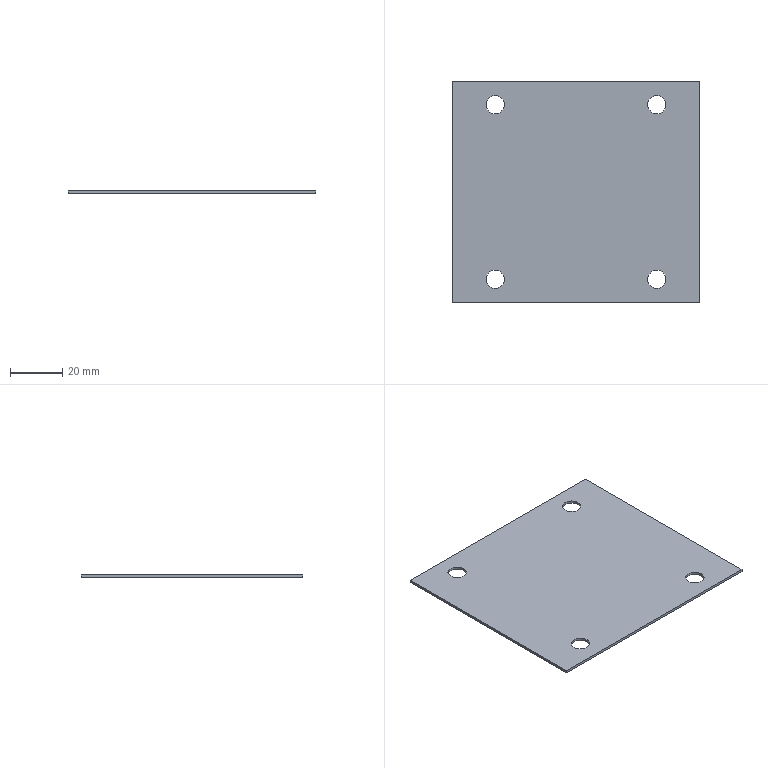Part | STEP file | GLSJ-10-45 | 1 solid | 14 faces | box 95 x 85 x 1 mm | volume 7921 mm3 | cylinder 8 | plane 6 | commonest cylinder face diameters 7 x8
STEP:
#1=CARTESIAN_POINT('',(0.,0.,0.));
#2=DIRECTION('',(0.,0.,1.));
#3=DIRECTION('',(1.,0.,0.));
#4=AXIS2_PLACEMENT_3D('',#1,#2,#3);
#5=CARTESIAN_POINT('',(-27.5,-33.5,0.));
#6=VERTEX_POINT('',#5);
#7=CARTESIAN_POINT('',(-27.5,-33.5,1.));
#8=VERTEX_POINT('',#7);
#9=CARTESIAN_POINT('',(-27.5,-33.5,0.));
#10=DIRECTION('',(0.,0.,1.));
#11=VECTOR('',#10,1.);
#12=LINE('',#9,#11);
#13=CARTESIAN_POINT('',(-31.,-33.5,0.));
#14=DIRECTION('',(0.,0.,1.));
#15=DIRECTION('',(1.,0.,0.));
#16=AXIS2_PLACEMENT_3D('',#13,#14,#15);
#17=CYLINDRICAL_SURFACE('',#16,3.5);
#18=CARTESIAN_POINT('',(6.283,0.));
#19=DIRECTION('',(0.,1.));
#20=VECTOR('',#19,1.);
#21=LINE('',#18,#20);
#22=(GEOMETRIC_REPRESENTATION_CONTEXT(2)PARAMETRIC_REPRESENTATION_CONTEXT()REPRESENTATION_CONTEXT('',''));
#23=DEFINITIONAL_REPRESENTATION('',(#21),#22);
#24=PCURVE('',#17,#23);
#25=CARTESIAN_POINT('',(-31.,-33.5,0.));
#26=DIRECTION('',(0.,0.,1.));
#27=DIRECTION('',(1.,0.,0.));
#28=AXIS2_PLACEMENT_3D('',#25,#26,#27);
#29=CYLINDRICAL_SURFACE('',#28,3.5);
#30=CARTESIAN_POINT('',(0.,0.));
#31=DIRECTION('',(0.,1.));
#32=VECTOR('',#31,1.);
#33=LINE('',#30,#32);
#34=(GEOMETRIC_REPRESENTATION_CONTEXT(2)PARAMETRIC_REPRESENTATION_CONTEXT()REPRESENTATION_CONTEXT('',''));
#35=DEFINITIONAL_REPRESENTATION('',(#33),#34);
#36=PCURVE('',#29,#35);
#37=SURFACE_CURVE('',#12,(#24,#36),.PCURVE_S1.);
#38=EDGE_CURVE('',#6,#8,#37,.T.);
#39=ORIENTED_EDGE('',*,*,#38,.T.);
#40=CARTESIAN_POINT('',(-34.5,-33.5,1.));
#41=VERTEX_POINT('',#40);
#42=CARTESIAN_POINT('',(-31.,-33.5,1.));
#43=DIRECTION('',(0.,0.,1.));
#44=DIRECTION('',(-1.,0.,0.));
#45=AXIS2_PLACEMENT_3D('',#42,#43,#44);
#46=CIRCLE('',#45,3.5);
#47=CARTESIAN_POINT('',(3.142,1.));
#48=DIRECTION('',(1.,0.));
#49=VECTOR('',#48,1.);
#50=LINE('',#47,#49);
#51=(GEOMETRIC_REPRESENTATION_CONTEXT(2)PARAMETRIC_REPRESENTATION_CONTEXT()REPRESENTATION_CONTEXT('',''));
#52=DEFINITIONAL_REPRESENTATION('',(#50),#51);
#53=PCURVE('',#17,#52);
#54=CARTESIAN_POINT('',(0.,0.,1.));
#55=DIRECTION('',(0.,0.,-1.));
#56=DIRECTION('',(-1.,0.,0.));
#57=AXIS2_PLACEMENT_3D('',#54,#55,#56);
#58=PLANE('',#57);
#59=CARTESIAN_POINT('',(34.5,-33.5));
#60=CARTESIAN_POINT('',(34.5,-39.562));
#61=CARTESIAN_POINT('',(29.25,-36.531));
#62=CARTESIAN_POINT('',(24.,-33.5));
#63=CARTESIAN_POINT('',(29.25,-30.469));
#64=CARTESIAN_POINT('',(34.5,-27.438));
#65=CARTESIAN_POINT('',(34.5,-33.5));
#66=(BOUNDED_CURVE()B_SPLINE_CURVE(2,(#59,#60,#61,#62,#63,#64,#65),.UNSPECIFIED.,.T.,.F.)B_SPLINE_CURVE_WITH_KNOTS((1,2,2,2,2,1),(-2.094,0.,2.094,4.189,6.283,8.378),.UNSPECIFIED.)CURVE()GEOMETRIC_REPRESENTATION_ITEM()RATIONAL_B_SPLINE_CURVE((1.,0.5,1.,0.5,1.,0.5,1.))REPRESENTATION_ITEM(''));
#67=(GEOMETRIC_REPRESENTATION_CONTEXT(2)PARAMETRIC_REPRESENTATION_CONTEXT()REPRESENTATION_CONTEXT('',''));
#68=DEFINITIONAL_REPRESENTATION('',(#66),#67);
#69=PCURVE('',#58,#68);
#70=SURFACE_CURVE('',#46,(#53,#69),.PCURVE_S1.);
#71=EDGE_CURVE('',#41,#8,#70,.T.);
#72=ORIENTED_EDGE('',*,*,#71,.F.);
#73=CARTESIAN_POINT('',(-34.5,-33.5,0.));
#74=VERTEX_POINT('',#73);
#75=CARTESIAN_POINT('',(-34.5,-33.5,0.));
#76=DIRECTION('',(0.,0.,1.));
#77=VECTOR('',#76,1.);
#78=LINE('',#75,#77);
#79=CARTESIAN_POINT('',(3.142,0.));
#80=DIRECTION('',(0.,1.));
#81=VECTOR('',#80,1.);
#82=LINE('',#79,#81);
#83=(GEOMETRIC_REPRESENTATION_CONTEXT(2)PARAMETRIC_REPRESENTATION_CONTEXT()REPRESENTATION_CONTEXT('',''));
#84=DEFINITIONAL_REPRESENTATION('',(#82),#83);
#85=PCURVE('',#17,#84);
#86=CARTESIAN_POINT('',(3.142,0.));
#87=DIRECTION('',(0.,1.));
#88=VECTOR('',#87,1.);
#89=LINE('',#86,#88);
#90=(GEOMETRIC_REPRESENTATION_CONTEXT(2)PARAMETRIC_REPRESENTATION_CONTEXT()REPRESENTATION_CONTEXT('',''));
#91=DEFINITIONAL_REPRESENTATION('',(#89),#90);
#92=PCURVE('',#29,#91);
#93=SURFACE_CURVE('',#78,(#85,#92),.PCURVE_S1.);
#94=EDGE_CURVE('',#74,#41,#93,.T.);
#95=ORIENTED_EDGE('',*,*,#94,.F.);
#96=CARTESIAN_POINT('',(-31.,-33.5,0.));
#97=DIRECTION('',(0.,0.,1.));
#98=DIRECTION('',(-1.,0.,0.));
#99=AXIS2_PLACEMENT_3D('',#96,#97,#98);
#100=CIRCLE('',#99,3.5);
#101=CARTESIAN_POINT('',(3.142,0.));
#102=DIRECTION('',(1.,0.));
#103=VECTOR('',#102,1.);
#104=LINE('',#101,#103);
#105=(GEOMETRIC_REPRESENTATION_CONTEXT(2)PARAMETRIC_REPRESENTATION_CONTEXT()REPRESENTATION_CONTEXT('',''));
#106=DEFINITIONAL_REPRESENTATION('',(#104),#105);
#107=PCURVE('',#17,#106);
#108=CARTESIAN_POINT('',(0.,0.,0.));
#109=DIRECTION('',(0.,0.,-1.));
#110=DIRECTION('',(-1.,0.,0.));
#111=AXIS2_PLACEMENT_3D('',#108,#109,#110);
#112=PLANE('',#111);
#113=CARTESIAN_POINT('',(34.5,-33.5));
#114=CARTESIAN_POINT('',(34.5,-39.562));
#115=CARTESIAN_POINT('',(29.25,-36.531));
#116=CARTESIAN_POINT('',(24.,-33.5));
#117=CARTESIAN_POINT('',(29.25,-30.469));
#118=CARTESIAN_POINT('',(34.5,-27.438));
#119=CARTESIAN_POINT('',(34.5,-33.5));
#120=(BOUNDED_CURVE()B_SPLINE_CURVE(2,(#113,#114,#115,#116,#117,#118,#119),.UNSPECIFIED.,.T.,.F.)B_SPLINE_CURVE_WITH_KNOTS((1,2,2,2,2,1),(-2.094,0.,2.094,4.189,6.283,8.378),.UNSPECIFIED.)CURVE()GEOMETRIC_REPRESENTATION_ITEM()RATIONAL_B_SPLINE_CURVE((1.,0.5,1.,0.5,1.,0.5,1.))REPRESENTATION_ITEM(''));
#121=(GEOMETRIC_REPRESENTATION_CONTEXT(2)PARAMETRIC_REPRESENTATION_CONTEXT()REPRESENTATION_CONTEXT('',''));
#122=DEFINITIONAL_REPRESENTATION('',(#120),#121);
#123=PCURVE('',#112,#122);
#124=SURFACE_CURVE('',#100,(#107,#123),.PCURVE_S1.);
#125=EDGE_CURVE('',#74,#6,#124,.T.);
#126=ORIENTED_EDGE('',*,*,#125,.T.);
#127=EDGE_LOOP('',(#39,#72,#95,#126));
#128=FACE_BOUND('',#127,.F.);
#129=ADVANCED_FACE('',(#128),#17,.F.);
#130=CARTESIAN_POINT('',(34.5,-33.5,0.));
#131=VERTEX_POINT('',#130);
#132=CARTESIAN_POINT('',(34.5,-33.5,1.));
#133=VERTEX_POINT('',#132);
#134=CARTESIAN_POINT('',(34.5,-33.5,0.));
#135=DIRECTION('',(0.,0.,1.));
#136=VECTOR('',#135,1.);
#137=LINE('',#134,#136);
#138=CARTESIAN_POINT('',(31.,-33.5,0.));
#139=DIRECTION('',(0.,0.,1.));
#140=DIRECTION('',(1.,0.,0.));
#141=AXIS2_PLACEMENT_3D('',#138,#139,#140);
#142=CYLINDRICAL_SURFACE('',#141,3.5);
#143=CARTESIAN_POINT('',(6.283,0.));
#144=DIRECTION('',(0.,1.));
#145=VECTOR('',#144,1.);
#146=LINE('',#143,#145);
#147=(GEOMETRIC_REPRESENTATION_CONTEXT(2)PARAMETRIC_REPRESENTATION_CONTEXT()REPRESENTATION_CONTEXT('',''));
#148=DEFINITIONAL_REPRESENTATION('',(#146),#147);
#149=PCURVE('',#142,#148);
#150=CARTESIAN_POINT('',(31.,-33.5,0.));
#151=DIRECTION('',(0.,0.,1.));
#152=DIRECTION('',(1.,0.,0.));
#153=AXIS2_PLACEMENT_3D('',#150,#151,#152);
#154=CYLINDRICAL_SURFACE('',#153,3.5);
#155=CARTESIAN_POINT('',(0.,0.));
#156=DIRECTION('',(0.,1.));
#157=VECTOR('',#156,1.);
#158=LINE('',#155,#157);
#159=(GEOMETRIC_REPRESENTATION_CONTEXT(2)PARAMETRIC_REPRESENTATION_CONTEXT()REPRESENTATION_CONTEXT('',''));
#160=DEFINITIONAL_REPRESENTATION('',(#158),#159);
#161=PCURVE('',#154,#160);
#162=SURFACE_CURVE('',#137,(#149,#161),.PCURVE_S1.);
#163=EDGE_CURVE('',#131,#133,#162,.T.);
#164=ORIENTED_EDGE('',*,*,#163,.T.);
#165=CARTESIAN_POINT('',(27.5,-33.5,1.));
#166=VERTEX_POINT('',#165);
#167=CARTESIAN_POINT('',(31.,-33.5,1.));
#168=DIRECTION('',(0.,0.,1.));
#169=DIRECTION('',(1.,0.,0.));
#170=AXIS2_PLACEMENT_3D('',#167,#168,#169);
#171=CIRCLE('',#170,3.5);
#172=CARTESIAN_POINT('',(0.,1.));
#173=DIRECTION('',(1.,0.));
#174=VECTOR('',#173,1.);
#175=LINE('',#172,#174);
#176=(GEOMETRIC_REPRESENTATION_CONTEXT(2)PARAMETRIC_REPRESENTATION_CONTEXT()REPRESENTATION_CONTEXT('',''));
#177=DEFINITIONAL_REPRESENTATION('',(#175),#176);
#178=PCURVE('',#142,#177);
#179=CARTESIAN_POINT('',(-34.5,-33.5));
#180=CARTESIAN_POINT('',(-34.5,-27.438));
#181=CARTESIAN_POINT('',(-29.25,-30.469));
#182=CARTESIAN_POINT('',(-24.,-33.5));
#183=CARTESIAN_POINT('',(-29.25,-36.531));
#184=CARTESIAN_POINT('',(-34.5,-39.562));
#185=CARTESIAN_POINT('',(-34.5,-33.5));
#186=(BOUNDED_CURVE()B_SPLINE_CURVE(2,(#179,#180,#181,#182,#183,#184,#185),.UNSPECIFIED.,.T.,.F.)B_SPLINE_CURVE_WITH_KNOTS((1,2,2,2,2,1),(-2.094,0.,2.094,4.189,6.283,8.378),.UNSPECIFIED.)CURVE()GEOMETRIC_REPRESENTATION_ITEM()RATIONAL_B_SPLINE_CURVE((1.,0.5,1.,0.5,1.,0.5,1.))REPRESENTATION_ITEM(''));
#187=(GEOMETRIC_REPRESENTATION_CONTEXT(2)PARAMETRIC_REPRESENTATION_CONTEXT()REPRESENTATION_CONTEXT('',''));
#188=DEFINITIONAL_REPRESENTATION('',(#186),#187);
#189=PCURVE('',#58,#188);
#190=SURFACE_CURVE('',#171,(#178,#189),.PCURVE_S1.);
#191=EDGE_CURVE('',#166,#133,#190,.T.);
#192=ORIENTED_EDGE('',*,*,#191,.F.);
#193=CARTESIAN_POINT('',(27.5,-33.5,0.));
#194=VERTEX_POINT('',#193);
#195=CARTESIAN_POINT('',(27.5,-33.5,0.));
#196=DIRECTION('',(0.,0.,1.));
#197=VECTOR('',#196,1.);
#198=LINE('',#195,#197);
#199=CARTESIAN_POINT('',(3.142,0.));
#200=DIRECTION('',(0.,1.));
#201=VECTOR('',#200,1.);
#202=LINE('',#199,#201);
#203=(GEOMETRIC_REPRESENTATION_CONTEXT(2)PARAMETRIC_REPRESENTATION_CONTEXT()REPRESENTATION_CONTEXT('',''));
#204=DEFINITIONAL_REPRESENTATION('',(#202),#203);
#205=PCURVE('',#142,#204);
#206=CARTESIAN_POINT('',(3.142,0.));
#207=DIRECTION('',(0.,1.));
#208=VECTOR('',#207,1.);
#209=LINE('',#206,#208);
#210=(GEOMETRIC_REPRESENTATION_CONTEXT(2)PARAMETRIC_REPRESENTATION_CONTEXT()REPRESENTATION_CONTEXT('',''));
#211=DEFINITIONAL_REPRESENTATION('',(#209),#210);
#212=PCURVE('',#154,#211);
#213=SURFACE_CURVE('',#198,(#205,#212),.PCURVE_S1.);
#214=EDGE_CURVE('',#194,#166,#213,.T.);
#215=ORIENTED_EDGE('',*,*,#214,.F.);
#216=CARTESIAN_POINT('',(31.,-33.5,0.));
#217=DIRECTION('',(0.,0.,1.));
#218=DIRECTION('',(1.,0.,0.));
#219=AXIS2_PLACEMENT_3D('',#216,#217,#218);
#220=CIRCLE('',#219,3.5);
#221=CARTESIAN_POINT('',(0.,0.));
#222=DIRECTION('',(1.,0.));
#223=VECTOR('',#222,1.);
#224=LINE('',#221,#223);
#225=(GEOMETRIC_REPRESENTATION_CONTEXT(2)PARAMETRIC_REPRESENTATION_CONTEXT()REPRESENTATION_CONTEXT('',''));
#226=DEFINITIONAL_REPRESENTATION('',(#224),#225);
#227=PCURVE('',#142,#226);
#228=CARTESIAN_POINT('',(-34.5,-33.5));
#229=CARTESIAN_POINT('',(-34.5,-27.438));
#230=CARTESIAN_POINT('',(-29.25,-30.469));
#231=CARTESIAN_POINT('',(-24.,-33.5));
#232=CARTESIAN_POINT('',(-29.25,-36.531));
#233=CARTESIAN_POINT('',(-34.5,-39.562));
#234=CARTESIAN_POINT('',(-34.5,-33.5));
#235=(BOUNDED_CURVE()B_SPLINE_CURVE(2,(#228,#229,#230,#231,#232,#233,#234),.UNSPECIFIED.,.T.,.F.)B_SPLINE_CURVE_WITH_KNOTS((1,2,2,2,2,1),(-2.094,0.,2.094,4.189,6.283,8.378),.UNSPECIFIED.)CURVE()GEOMETRIC_REPRESENTATION_ITEM()RATIONAL_B_SPLINE_CURVE((1.,0.5,1.,0.5,1.,0.5,1.))REPRESENTATION_ITEM(''));
#236=(GEOMETRIC_REPRESENTATION_CONTEXT(2)PARAMETRIC_REPRESENTATION_CONTEXT()REPRESENTATION_CONTEXT('',''));
#237=DEFINITIONAL_REPRESENTATION('',(#235),#236);
#238=PCURVE('',#112,#237);
#239=SURFACE_CURVE('',#220,(#227,#238),.PCURVE_S1.);
#240=EDGE_CURVE('',#194,#131,#239,.T.);
#241=ORIENTED_EDGE('',*,*,#240,.T.);
#242=EDGE_LOOP('',(#164,#192,#215,#241));
#243=FACE_BOUND('',#242,.F.);
#244=ADVANCED_FACE('',(#243),#142,.F.);
#245=CARTESIAN_POINT('',(34.5,33.5,0.));
#246=VERTEX_POINT('',#245);
#247=CARTESIAN_POINT('',(34.5,33.5,1.));
#248=VERTEX_POINT('',#247);
#249=CARTESIAN_POINT('',(34.5,33.5,0.));
#250=DIRECTION('',(0.,0.,1.));
#251=VECTOR('',#250,1.);
#252=LINE('',#249,#251);
#253=CARTESIAN_POINT('',(31.,33.5,0.));
#254=DIRECTION('',(0.,0.,1.));
#255=DIRECTION('',(1.,0.,0.));
#256=AXIS2_PLACEMENT_3D('',#253,#254,#255);
#257=CYLINDRICAL_SURFACE('',#256,3.5);
#258=CARTESIAN_POINT('',(6.283,0.));
#259=DIRECTION('',(0.,1.));
#260=VECTOR('',#259,1.);
#261=LINE('',#258,#260);
#262=(GEOMETRIC_REPRESENTATION_CONTEXT(2)PARAMETRIC_REPRESENTATION_CONTEXT()REPRESENTATION_CONTEXT('',''));
#263=DEFINITIONAL_REPRESENTATION('',(#261),#262);
#264=PCURVE('',#257,#263);
#265=CARTESIAN_POINT('',(31.,33.5,0.));
#266=DIRECTION('',(0.,0.,1.));
#267=DIRECTION('',(1.,0.,0.));
#268=AXIS2_PLACEMENT_3D('',#265,#266,#267);
#269=CYLINDRICAL_SURFACE('',#268,3.5);
#270=CARTESIAN_POINT('',(0.,0.));
#271=DIRECTION('',(0.,1.));
#272=VECTOR('',#271,1.);
#273=LINE('',#270,#272);
#274=(GEOMETRIC_REPRESENTATION_CONTEXT(2)PARAMETRIC_REPRESENTATION_CONTEXT()REPRESENTATION_CONTEXT('',''));
#275=DEFINITIONAL_REPRESENTATION('',(#273),#274);
#276=PCURVE('',#269,#275);
#277=SURFACE_CURVE('',#252,(#264,#276),.PCURVE_S1.);
#278=EDGE_CURVE('',#246,#248,#277,.T.);
#279=ORIENTED_EDGE('',*,*,#278,.T.);
#280=CARTESIAN_POINT('',(27.5,33.5,1.));
#281=VERTEX_POINT('',#280);
#282=CARTESIAN_POINT('',(31.,33.5,1.));
#283=DIRECTION('',(0.,0.,1.));
#284=DIRECTION('',(-1.,0.,0.));
#285=AXIS2_PLACEMENT_3D('',#282,#283,#284);
#286=CIRCLE('',#285,3.5);
#287=CARTESIAN_POINT('',(3.142,1.));
#288=DIRECTION('',(1.,0.));
#289=VECTOR('',#288,1.);
#290=LINE('',#287,#289);
#291=(GEOMETRIC_REPRESENTATION_CONTEXT(2)PARAMETRIC_REPRESENTATION_CONTEXT()REPRESENTATION_CONTEXT('',''));
#292=DEFINITIONAL_REPRESENTATION('',(#290),#291);
#293=PCURVE('',#257,#292);
#294=CARTESIAN_POINT('',(-27.5,33.5));
#295=CARTESIAN_POINT('',(-27.5,27.438));
#296=CARTESIAN_POINT('',(-32.75,30.469));
#297=CARTESIAN_POINT('',(-38.,33.5));
#298=CARTESIAN_POINT('',(-32.75,36.531));
#299=CARTESIAN_POINT('',(-27.5,39.562));
#300=CARTESIAN_POINT('',(-27.5,33.5));
#301=(BOUNDED_CURVE()B_SPLINE_CURVE(2,(#294,#295,#296,#297,#298,#299,#300),.UNSPECIFIED.,.T.,.F.)B_SPLINE_CURVE_WITH_KNOTS((1,2,2,2,2,1),(-2.094,0.,2.094,4.189,6.283,8.378),.UNSPECIFIED.)CURVE()GEOMETRIC_REPRESENTATION_ITEM()RATIONAL_B_SPLINE_CURVE((1.,0.5,1.,0.5,1.,0.5,1.))REPRESENTATION_ITEM(''));
#302=(GEOMETRIC_REPRESENTATION_CONTEXT(2)PARAMETRIC_REPRESENTATION_CONTEXT()REPRESENTATION_CONTEXT('',''));
#303=DEFINITIONAL_REPRESENTATION('',(#301),#302);
#304=PCURVE('',#58,#303);
#305=SURFACE_CURVE('',#286,(#293,#304),.PCURVE_S1.);
#306=EDGE_CURVE('',#281,#248,#305,.T.);
#307=ORIENTED_EDGE('',*,*,#306,.F.);
#308=CARTESIAN_POINT('',(27.5,33.5,0.));
#309=VERTEX_POINT('',#308);
#310=CARTESIAN_POINT('',(27.5,33.5,0.));
#311=DIRECTION('',(0.,0.,1.));
#312=VECTOR('',#311,1.);
#313=LINE('',#310,#312);
#314=CARTESIAN_POINT('',(3.142,0.));
#315=DIRECTION('',(0.,1.));
#316=VECTOR('',#315,1.);
#317=LINE('',#314,#316);
#318=(GEOMETRIC_REPRESENTATION_CONTEXT(2)PARAMETRIC_REPRESENTATION_CONTEXT()REPRESENTATION_CONTEXT('',''));
#319=DEFINITIONAL_REPRESENTATION('',(#317),#318);
#320=PCURVE('',#257,#319);
#321=CARTESIAN_POINT('',(3.142,0.));
#322=DIRECTION('',(0.,1.));
#323=VECTOR('',#322,1.);
#324=LINE('',#321,#323);
#325=(GEOMETRIC_REPRESENTATION_CONTEXT(2)PARAMETRIC_REPRESENTATION_CONTEXT()REPRESENTATION_CONTEXT('',''));
#326=DEFINITIONAL_REPRESENTATION('',(#324),#325);
#327=PCURVE('',#269,#326);
#328=SURFACE_CURVE('',#313,(#320,#327),.PCURVE_S1.);
#329=EDGE_CURVE('',#309,#281,#328,.T.);
#330=ORIENTED_EDGE('',*,*,#329,.F.);
#331=CARTESIAN_POINT('',(31.,33.5,0.));
#332=DIRECTION('',(0.,0.,1.));
#333=DIRECTION('',(-1.,0.,0.));
#334=AXIS2_PLACEMENT_3D('',#331,#332,#333);
#335=CIRCLE('',#334,3.5);
#336=CARTESIAN_POINT('',(3.142,0.));
#337=DIRECTION('',(1.,0.));
#338=VECTOR('',#337,1.);
#339=LINE('',#336,#338);
#340=(GEOMETRIC_REPRESENTATION_CONTEXT(2)PARAMETRIC_REPRESENTATION_CONTEXT()REPRESENTATION_CONTEXT('',''));
#341=DEFINITIONAL_REPRESENTATION('',(#339),#340);
#342=PCURVE('',#257,#341);
#343=CARTESIAN_POINT('',(-27.5,33.5));
#344=CARTESIAN_POINT('',(-27.5,27.438));
#345=CARTESIAN_POINT('',(-32.75,30.469));
#346=CARTESIAN_POINT('',(-38.,33.5));
#347=CARTESIAN_POINT('',(-32.75,36.531));
#348=CARTESIAN_POINT('',(-27.5,39.562));
#349=CARTESIAN_POINT('',(-27.5,33.5));
#350=(BOUNDED_CURVE()B_SPLINE_CURVE(2,(#343,#344,#345,#346,#347,#348,#349),.UNSPECIFIED.,.T.,.F.)B_SPLINE_CURVE_WITH_KNOTS((1,2,2,2,2,1),(-2.094,0.,2.094,4.189,6.283,8.378),.UNSPECIFIED.)CURVE()GEOMETRIC_REPRESENTATION_ITEM()RATIONAL_B_SPLINE_CURVE((1.,0.5,1.,0.5,1.,0.5,1.))REPRESENTATION_ITEM(''));
#351=(GEOMETRIC_REPRESENTATION_CONTEXT(2)PARAMETRIC_REPRESENTATION_CONTEXT()REPRESENTATION_CONTEXT('',''));
#352=DEFINITIONAL_REPRESENTATION('',(#350),#351);
#353=PCURVE('',#112,#352);
#354=SURFACE_CURVE('',#335,(#342,#353),.PCURVE_S1.);
#355=EDGE_CURVE('',#309,#246,#354,.T.);
#356=ORIENTED_EDGE('',*,*,#355,.T.);
#357=EDGE_LOOP('',(#279,#307,#330,#356));
#358=FACE_BOUND('',#357,.F.);
#359=ADVANCED_FACE('',(#358),#257,.F.);
#360=CARTESIAN_POINT('',(-27.5,33.5,0.));
#361=VERTEX_POINT('',#360);
#362=CARTESIAN_POINT('',(-27.5,33.5,1.));
#363=VERTEX_POINT('',#362);
#364=CARTESIAN_POINT('',(-27.5,33.5,0.));
#365=DIRECTION('',(0.,0.,1.));
#366=VECTOR('',#365,1.);
#367=LINE('',#364,#366);
#368=CARTESIAN_POINT('',(-31.,33.5,0.));
#369=DIRECTION('',(0.,0.,1.));
#370=DIRECTION('',(1.,0.,0.));
#371=AXIS2_PLACEMENT_3D('',#368,#369,#370);
#372=CYLINDRICAL_SURFACE('',#371,3.5);
#373=CARTESIAN_POINT('',(6.283,0.));
#374=DIRECTION('',(0.,1.));
#375=VECTOR('',#374,1.);
#376=LINE('',#373,#375);
#377=(GEOMETRIC_REPRESENTATION_CONTEXT(2)PARAMETRIC_REPRESENTATION_CONTEXT()REPRESENTATION_CONTEXT('',''));
#378=DEFINITIONAL_REPRESENTATION('',(#376),#377);
#379=PCURVE('',#372,#378);
#380=CARTESIAN_POINT('',(-31.,33.5,0.));
#381=DIRECTION('',(0.,0.,1.));
#382=DIRECTION('',(1.,0.,0.));
#383=AXIS2_PLACEMENT_3D('',#380,#381,#382);
#384=CYLINDRICAL_SURFACE('',#383,3.5);
#385=CARTESIAN_POINT('',(0.,0.));
#386=DIRECTION('',(0.,1.));
#387=VECTOR('',#386,1.);
#388=LINE('',#385,#387);
#389=(GEOMETRIC_REPRESENTATION_CONTEXT(2)PARAMETRIC_REPRESENTATION_CONTEXT()REPRESENTATION_CONTEXT('',''));
#390=DEFINITIONAL_REPRESENTATION('',(#388),#389);
#391=PCURVE('',#384,#390);
#392=SURFACE_CURVE('',#367,(#379,#391),.PCURVE_S1.);
#393=EDGE_CURVE('',#361,#363,#392,.T.);
#394=ORIENTED_EDGE('',*,*,#393,.T.);
#395=CARTESIAN_POINT('',(-34.5,33.5,1.));
#396=VERTEX_POINT('',#395);
#397=CARTESIAN_POINT('',(-31.,33.5,1.));
#398=DIRECTION('',(0.,0.,1.));
#399=DIRECTION('',(1.,0.,0.));
#400=AXIS2_PLACEMENT_3D('',#397,#398,#399);
#401=CIRCLE('',#400,3.5);
#402=CARTESIAN_POINT('',(0.,1.));
#403=DIRECTION('',(1.,0.));
#404=VECTOR('',#403,1.);
#405=LINE('',#402,#404);
#406=(GEOMETRIC_REPRESENTATION_CONTEXT(2)PARAMETRIC_REPRESENTATION_CONTEXT()REPRESENTATION_CONTEXT('',''));
#407=DEFINITIONAL_REPRESENTATION('',(#405),#406);
#408=PCURVE('',#372,#407);
#409=CARTESIAN_POINT('',(27.5,33.5));
#410=CARTESIAN_POINT('',(27.5,39.562));
#411=CARTESIAN_POINT('',(32.75,36.531));
#412=CARTESIAN_POINT('',(38.,33.5));
#413=CARTESIAN_POINT('',(32.75,30.469));
#414=CARTESIAN_POINT('',(27.5,27.438));
#415=CARTESIAN_POINT('',(27.5,33.5));
#416=(BOUNDED_CURVE()B_SPLINE_CURVE(2,(#409,#410,#411,#412,#413,#414,#415),.UNSPECIFIED.,.T.,.F.)B_SPLINE_CURVE_WITH_KNOTS((1,2,2,2,2,1),(-2.094,0.,2.094,4.189,6.283,8.378),.UNSPECIFIED.)CURVE()GEOMETRIC_REPRESENTATION_ITEM()RATIONAL_B_SPLINE_CURVE((1.,0.5,1.,0.5,1.,0.5,1.))REPRESENTATION_ITEM(''));
#417=(GEOMETRIC_REPRESENTATION_CONTEXT(2)PARAMETRIC_REPRESENTATION_CONTEXT()REPRESENTATION_CONTEXT('',''));
#418=DEFINITIONAL_REPRESENTATION('',(#416),#417);
#419=PCURVE('',#58,#418);
#420=SURFACE_CURVE('',#401,(#408,#419),.PCURVE_S1.);
#421=EDGE_CURVE('',#396,#363,#420,.T.);
#422=ORIENTED_EDGE('',*,*,#421,.F.);
#423=CARTESIAN_POINT('',(-34.5,33.5,0.));
#424=VERTEX_POINT('',#423);
#425=CARTESIAN_POINT('',(-34.5,33.5,0.));
#426=DIRECTION('',(0.,0.,1.));
#427=VECTOR('',#426,1.);
#428=LINE('',#425,#427);
#429=CARTESIAN_POINT('',(3.142,0.));
#430=DIRECTION('',(0.,1.));
#431=VECTOR('',#430,1.);
#432=LINE('',#429,#431);
#433=(GEOMETRIC_REPRESENTATION_CONTEXT(2)PARAMETRIC_REPRESENTATION_CONTEXT()REPRESENTATION_CONTEXT('',''));
#434=DEFINITIONAL_REPRESENTATION('',(#432),#433);
#435=PCURVE('',#372,#434);
#436=CARTESIAN_POINT('',(3.142,0.));
#437=DIRECTION('',(0.,1.));
#438=VECTOR('',#437,1.);
#439=LINE('',#436,#438);
#440=(GEOMETRIC_REPRESENTATION_CONTEXT(2)PARAMETRIC_REPRESENTATION_CONTEXT()REPRESENTATION_CONTEXT('',''));
#441=DEFINITIONAL_REPRESENTATION('',(#439),#440);
#442=PCURVE('',#384,#441);
#443=SURFACE_CURVE('',#428,(#435,#442),.PCURVE_S1.);
#444=EDGE_CURVE('',#424,#396,#443,.T.);
#445=ORIENTED_EDGE('',*,*,#444,.F.);
#446=CARTESIAN_POINT('',(-31.,33.5,0.));
#447=DIRECTION('',(0.,0.,1.));
#448=DIRECTION('',(1.,0.,0.));
#449=AXIS2_PLACEMENT_3D('',#446,#447,#448);
#450=CIRCLE('',#449,3.5);
#451=CARTESIAN_POINT('',(0.,0.));
#452=DIRECTION('',(1.,0.));
#453=VECTOR('',#452,1.);
#454=LINE('',#451,#453);
#455=(GEOMETRIC_REPRESENTATION_CONTEXT(2)PARAMETRIC_REPRESENTATION_CONTEXT()REPRESENTATION_CONTEXT('',''));
#456=DEFINITIONAL_REPRESENTATION('',(#454),#455);
#457=PCURVE('',#372,#456);
#458=CARTESIAN_POINT('',(27.5,33.5));
#459=CARTESIAN_POINT('',(27.5,39.562));
#460=CARTESIAN_POINT('',(32.75,36.531));
#461=CARTESIAN_POINT('',(38.,33.5));
#462=CARTESIAN_POINT('',(32.75,30.469));
#463=CARTESIAN_POINT('',(27.5,27.438));
#464=CARTESIAN_POINT('',(27.5,33.5));
#465=(BOUNDED_CURVE()B_SPLINE_CURVE(2,(#458,#459,#460,#461,#462,#463,#464),.UNSPECIFIED.,.T.,.F.)B_SPLINE_CURVE_WITH_KNOTS((1,2,2,2,2,1),(-2.094,0.,2.094,4.189,6.283,8.378),.UNSPECIFIED.)CURVE()GEOMETRIC_REPRESENTATION_ITEM()RATIONAL_B_SPLINE_CURVE((1.,0.5,1.,0.5,1.,0.5,1.))REPRESENTATION_ITEM(''));
#466=(GEOMETRIC_REPRESENTATION_CONTEXT(2)PARAMETRIC_REPRESENTATION_CONTEXT()REPRESENTATION_CONTEXT('',''));
#467=DEFINITIONAL_REPRESENTATION('',(#465),#466);
#468=PCURVE('',#112,#467);
#469=SURFACE_CURVE('',#450,(#457,#468),.PCURVE_S1.);
#470=EDGE_CURVE('',#424,#361,#469,.T.);
#471=ORIENTED_EDGE('',*,*,#470,.T.);
#472=EDGE_LOOP('',(#394,#422,#445,#471));
#473=FACE_BOUND('',#472,.F.);
#474=ADVANCED_FACE('',(#473),#372,.F.);
#475=CARTESIAN_POINT('',(-47.5,42.5,0.));
#476=VERTEX_POINT('',#475);
#477=CARTESIAN_POINT('',(-47.5,-42.5,0.));
#478=VERTEX_POINT('',#477);
#479=CARTESIAN_POINT('',(-47.5,42.5,0.));
#480=DIRECTION('',(0.,-1.,0.));
#481=VECTOR('',#480,1.);
#482=LINE('',#479,#481);
#483=CARTESIAN_POINT('',(-47.5,42.5,1.));
#484=DIRECTION('',(1.,0.,0.));
#485=DIRECTION('',(0.,1.,0.));
#486=AXIS2_PLACEMENT_3D('',#483,#484,#485);
#487=PLANE('',#486);
#488=CARTESIAN_POINT('',(0.,-1.));
#489=DIRECTION('',(-1.,0.));
#490=VECTOR('',#489,1.);
#491=LINE('',#488,#490);
#492=(GEOMETRIC_REPRESENTATION_CONTEXT(2)PARAMETRIC_REPRESENTATION_CONTEXT()REPRESENTATION_CONTEXT('',''));
#493=DEFINITIONAL_REPRESENTATION('',(#491),#492);
#494=PCURVE('',#487,#493);
#495=CARTESIAN_POINT('',(47.5,42.5));
#496=DIRECTION('',(0.,-1.));
#497=VECTOR('',#496,1.);
#498=LINE('',#495,#497);
#499=(GEOMETRIC_REPRESENTATION_CONTEXT(2)PARAMETRIC_REPRESENTATION_CONTEXT()REPRESENTATION_CONTEXT('',''));
#500=DEFINITIONAL_REPRESENTATION('',(#498),#499);
#501=PCURVE('',#112,#500);
#502=SURFACE_CURVE('',#482,(#494,#501),.PCURVE_S1.);
#503=EDGE_CURVE('',#476,#478,#502,.T.);
#504=ORIENTED_EDGE('',*,*,#503,.T.);
#505=CARTESIAN_POINT('',(-47.5,-42.5,1.));
#506=VERTEX_POINT('',#505);
#507=CARTESIAN_POINT('',(-47.5,-42.5,1.));
#508=DIRECTION('',(0.,0.,-1.));
#509=VECTOR('',#508,1.);
#510=LINE('',#507,#509);
#511=CARTESIAN_POINT('',(-85.,0.));
#512=DIRECTION('',(0.,-1.));
#513=VECTOR('',#512,1.);
#514=LINE('',#511,#513);
#515=(GEOMETRIC_REPRESENTATION_CONTEXT(2)PARAMETRIC_REPRESENTATION_CONTEXT()REPRESENTATION_CONTEXT('',''));
#516=DEFINITIONAL_REPRESENTATION('',(#514),#515);
#517=PCURVE('',#487,#516);
#518=CARTESIAN_POINT('',(47.5,-42.5,1.));
#519=DIRECTION('',(0.,1.,0.));
#520=DIRECTION('',(-1.,0.,0.));
#521=AXIS2_PLACEMENT_3D('',#518,#519,#520);
#522=PLANE('',#521);
#523=CARTESIAN_POINT('',(95.,0.));
#524=DIRECTION('',(0.,-1.));
#525=VECTOR('',#524,1.);
#526=LINE('',#523,#525);
#527=(GEOMETRIC_REPRESENTATION_CONTEXT(2)PARAMETRIC_REPRESENTATION_CONTEXT()REPRESENTATION_CONTEXT('',''));
#528=DEFINITIONAL_REPRESENTATION('',(#526),#527);
#529=PCURVE('',#522,#528);
#530=SURFACE_CURVE('',#510,(#517,#529),.PCURVE_S1.);
#531=EDGE_CURVE('',#506,#478,#530,.T.);
#532=ORIENTED_EDGE('',*,*,#531,.F.);
#533=CARTESIAN_POINT('',(-47.5,42.5,1.));
#534=VERTEX_POINT('',#533);
#535=CARTESIAN_POINT('',(-47.5,42.5,1.));
#536=DIRECTION('',(0.,-1.,0.));
#537=VECTOR('',#536,1.);
#538=LINE('',#535,#537);
#539=CARTESIAN_POINT('',(0.,0.));
#540=DIRECTION('',(-1.,0.));
#541=VECTOR('',#540,1.);
#542=LINE('',#539,#541);
#543=(GEOMETRIC_REPRESENTATION_CONTEXT(2)PARAMETRIC_REPRESENTATION_CONTEXT()REPRESENTATION_CONTEXT('',''));
#544=DEFINITIONAL_REPRESENTATION('',(#542),#543);
#545=PCURVE('',#487,#544);
#546=CARTESIAN_POINT('',(47.5,42.5));
#547=DIRECTION('',(0.,-1.));
#548=VECTOR('',#547,1.);
#549=LINE('',#546,#548);
#550=(GEOMETRIC_REPRESENTATION_CONTEXT(2)PARAMETRIC_REPRESENTATION_CONTEXT()REPRESENTATION_CONTEXT('',''));
#551=DEFINITIONAL_REPRESENTATION('',(#549),#550);
#552=PCURVE('',#58,#551);
#553=SURFACE_CURVE('',#538,(#545,#552),.PCURVE_S1.);
#554=EDGE_CURVE('',#534,#506,#553,.T.);
#555=ORIENTED_EDGE('',*,*,#554,.F.);
#556=CARTESIAN_POINT('',(-47.5,42.5,1.));
#557=DIRECTION('',(0.,0.,-1.));
#558=VECTOR('',#557,1.);
#559=LINE('',#556,#558);
#560=CARTESIAN_POINT('',(0.,0.));
#561=DIRECTION('',(0.,-1.));
#562=VECTOR('',#561,1.);
#563=LINE('',#560,#562);
#564=(GEOMETRIC_REPRESENTATION_CONTEXT(2)PARAMETRIC_REPRESENTATION_CONTEXT()REPRESENTATION_CONTEXT('',''));
#565=DEFINITIONAL_REPRESENTATION('',(#563),#564);
#566=PCURVE('',#487,#565);
#567=CARTESIAN_POINT('',(47.5,42.5,1.));
#568=DIRECTION('',(0.,-1.,0.));
#569=DIRECTION('',(1.,0.,0.));
#570=AXIS2_PLACEMENT_3D('',#567,#568,#569);
#571=PLANE('',#570);
#572=CARTESIAN_POINT('',(-95.,0.));
#573=DIRECTION('',(0.,-1.));
#574=VECTOR('',#573,1.);
#575=LINE('',#572,#574);
#576=(GEOMETRIC_REPRESENTATION_CONTEXT(2)PARAMETRIC_REPRESENTATION_CONTEXT()REPRESENTATION_CONTEXT('',''));
#577=DEFINITIONAL_REPRESENTATION('',(#575),#576);
#578=PCURVE('',#571,#577);
#579=SURFACE_CURVE('',#559,(#566,#578),.PCURVE_S1.);
#580=EDGE_CURVE('',#534,#476,#579,.T.);
#581=ORIENTED_EDGE('',*,*,#580,.T.);
#582=EDGE_LOOP('',(#504,#532,#555,#581));
#583=FACE_BOUND('',#582,.T.);
#584=ADVANCED_FACE('',(#583),#487,.F.);
#585=CARTESIAN_POINT('',(47.5,-42.5,0.));
#586=VERTEX_POINT('',#585);
#587=CARTESIAN_POINT('',(47.5,-42.5,0.));
#588=DIRECTION('',(1.,0.,0.));
#589=VECTOR('',#588,1.);
#590=LINE('',#587,#589);
#591=CARTESIAN_POINT('',(0.,-1.));
#592=DIRECTION('',(-1.,0.));
#593=VECTOR('',#592,1.);
#594=LINE('',#591,#593);
#595=(GEOMETRIC_REPRESENTATION_CONTEXT(2)PARAMETRIC_REPRESENTATION_CONTEXT()REPRESENTATION_CONTEXT('',''));
#596=DEFINITIONAL_REPRESENTATION('',(#594),#595);
#597=PCURVE('',#522,#596);
#598=CARTESIAN_POINT('',(-47.5,-42.5));
#599=DIRECTION('',(-1.,0.));
#600=VECTOR('',#599,1.);
#601=LINE('',#598,#600);
#602=(GEOMETRIC_REPRESENTATION_CONTEXT(2)PARAMETRIC_REPRESENTATION_CONTEXT()REPRESENTATION_CONTEXT('',''));
#603=DEFINITIONAL_REPRESENTATION('',(#601),#602);
#604=PCURVE('',#112,#603);
#605=SURFACE_CURVE('',#590,(#597,#604),.PCURVE_S1.);
#606=EDGE_CURVE('',#478,#586,#605,.T.);
#607=ORIENTED_EDGE('',*,*,#606,.T.);
#608=CARTESIAN_POINT('',(47.5,-42.5,1.));
#609=VERTEX_POINT('',#608);
#610=CARTESIAN_POINT('',(47.5,-42.5,1.));
#611=DIRECTION('',(0.,0.,-1.));
#612=VECTOR('',#611,1.);
#613=LINE('',#610,#612);
#614=CARTESIAN_POINT('',(0.,0.));
#615=DIRECTION('',(0.,-1.));
#616=VECTOR('',#615,1.);
#617=LINE('',#614,#616);
#618=(GEOMETRIC_REPRESENTATION_CONTEXT(2)PARAMETRIC_REPRESENTATION_CONTEXT()REPRESENTATION_CONTEXT('',''));
#619=DEFINITIONAL_REPRESENTATION('',(#617),#618);
#620=PCURVE('',#522,#619);
#621=CARTESIAN_POINT('',(47.5,42.5,1.));
#622=DIRECTION('',(-1.,0.,0.));
#623=DIRECTION('',(0.,-1.,0.));
#624=AXIS2_PLACEMENT_3D('',#621,#622,#623);
#625=PLANE('',#624);
#626=CARTESIAN_POINT('',(85.,0.));
#627=DIRECTION('',(0.,-1.));
#628=VECTOR('',#627,1.);
#629=LINE('',#626,#628);
#630=(GEOMETRIC_REPRESENTATION_CONTEXT(2)PARAMETRIC_REPRESENTATION_CONTEXT()REPRESENTATION_CONTEXT('',''));
#631=DEFINITIONAL_REPRESENTATION('',(#629),#630);
#632=PCURVE('',#625,#631);
#633=SURFACE_CURVE('',#613,(#620,#632),.PCURVE_S1.);
#634=EDGE_CURVE('',#609,#586,#633,.T.);
#635=ORIENTED_EDGE('',*,*,#634,.F.);
#636=CARTESIAN_POINT('',(47.5,-42.5,1.));
#637=DIRECTION('',(1.,0.,0.));
#638=VECTOR('',#637,1.);
#639=LINE('',#636,#638);
#640=CARTESIAN_POINT('',(0.,0.));
#641=DIRECTION('',(-1.,0.));
#642=VECTOR('',#641,1.);
#643=LINE('',#640,#642);
#644=(GEOMETRIC_REPRESENTATION_CONTEXT(2)PARAMETRIC_REPRESENTATION_CONTEXT()REPRESENTATION_CONTEXT('',''));
#645=DEFINITIONAL_REPRESENTATION('',(#643),#644);
#646=PCURVE('',#522,#645);
#647=CARTESIAN_POINT('',(-47.5,-42.5));
#648=DIRECTION('',(-1.,0.));
#649=VECTOR('',#648,1.);
#650=LINE('',#647,#649);
#651=(GEOMETRIC_REPRESENTATION_CONTEXT(2)PARAMETRIC_REPRESENTATION_CONTEXT()REPRESENTATION_CONTEXT('',''));
#652=DEFINITIONAL_REPRESENTATION('',(#650),#651);
#653=PCURVE('',#58,#652);
#654=SURFACE_CURVE('',#639,(#646,#653),.PCURVE_S1.);
#655=EDGE_CURVE('',#506,#609,#654,.T.);
#656=ORIENTED_EDGE('',*,*,#655,.F.);
#657=ORIENTED_EDGE('',*,*,#531,.T.);
#658=EDGE_LOOP('',(#607,#635,#656,#657));
#659=FACE_BOUND('',#658,.T.);
#660=ADVANCED_FACE('',(#659),#522,.F.);
#661=CARTESIAN_POINT('',(47.5,42.5,0.));
#662=VERTEX_POINT('',#661);
#663=CARTESIAN_POINT('',(47.5,42.5,0.));
#664=DIRECTION('',(0.,1.,0.));
#665=VECTOR('',#664,1.);
#666=LINE('',#663,#665);
#667=CARTESIAN_POINT('',(0.,-1.));
#668=DIRECTION('',(-1.,0.));
#669=VECTOR('',#668,1.);
#670=LINE('',#667,#669);
#671=(GEOMETRIC_REPRESENTATION_CONTEXT(2)PARAMETRIC_REPRESENTATION_CONTEXT()REPRESENTATION_CONTEXT('',''));
#672=DEFINITIONAL_REPRESENTATION('',(#670),#671);
#673=PCURVE('',#625,#672);
#674=CARTESIAN_POINT('',(-47.5,42.5));
#675=DIRECTION('',(0.,1.));
#676=VECTOR('',#675,1.);
#677=LINE('',#674,#676);
#678=(GEOMETRIC_REPRESENTATION_CONTEXT(2)PARAMETRIC_REPRESENTATION_CONTEXT()REPRESENTATION_CONTEXT('',''));
#679=DEFINITIONAL_REPRESENTATION('',(#677),#678);
#680=PCURVE('',#112,#679);
#681=SURFACE_CURVE('',#666,(#673,#680),.PCURVE_S1.);
#682=EDGE_CURVE('',#586,#662,#681,.T.);
#683=ORIENTED_EDGE('',*,*,#682,.T.);
#684=CARTESIAN_POINT('',(47.5,42.5,1.));
#685=VERTEX_POINT('',#684);
#686=CARTESIAN_POINT('',(47.5,42.5,1.));
#687=DIRECTION('',(0.,0.,-1.));
#688=VECTOR('',#687,1.);
#689=LINE('',#686,#688);
#690=CARTESIAN_POINT('',(0.,0.));
#691=DIRECTION('',(0.,-1.));
#692=VECTOR('',#691,1.);
#693=LINE('',#690,#692);
#694=(GEOMETRIC_REPRESENTATION_CONTEXT(2)PARAMETRIC_REPRESENTATION_CONTEXT()REPRESENTATION_CONTEXT('',''));
#695=DEFINITIONAL_REPRESENTATION('',(#693),#694);
#696=PCURVE('',#625,#695);
#697=CARTESIAN_POINT('',(0.,0.));
#698=DIRECTION('',(0.,-1.));
#699=VECTOR('',#698,1.);
#700=LINE('',#697,#699);
#701=(GEOMETRIC_REPRESENTATION_CONTEXT(2)PARAMETRIC_REPRESENTATION_CONTEXT()REPRESENTATION_CONTEXT('',''));
#702=DEFINITIONAL_REPRESENTATION('',(#700),#701);
#703=PCURVE('',#571,#702);
#704=SURFACE_CURVE('',#689,(#696,#703),.PCURVE_S1.);
#705=EDGE_CURVE('',#685,#662,#704,.T.);
#706=ORIENTED_EDGE('',*,*,#705,.F.);
#707=CARTESIAN_POINT('',(47.5,42.5,1.));
#708=DIRECTION('',(0.,1.,0.));
#709=VECTOR('',#708,1.);
#710=LINE('',#707,#709);
#711=CARTESIAN_POINT('',(0.,0.));
#712=DIRECTION('',(-1.,0.));
#713=VECTOR('',#712,1.);
#714=LINE('',#711,#713);
#715=(GEOMETRIC_REPRESENTATION_CONTEXT(2)PARAMETRIC_REPRESENTATION_CONTEXT()REPRESENTATION_CONTEXT('',''));
#716=DEFINITIONAL_REPRESENTATION('',(#714),#715);
#717=PCURVE('',#625,#716);
#718=CARTESIAN_POINT('',(-47.5,42.5));
#719=DIRECTION('',(0.,1.));
#720=VECTOR('',#719,1.);
#721=LINE('',#718,#720);
#722=(GEOMETRIC_REPRESENTATION_CONTEXT(2)PARAMETRIC_REPRESENTATION_CONTEXT()REPRESENTATION_CONTEXT('',''));
#723=DEFINITIONAL_REPRESENTATION('',(#721),#722);
#724=PCURVE('',#58,#723);
#725=SURFACE_CURVE('',#710,(#717,#724),.PCURVE_S1.);
#726=EDGE_CURVE('',#609,#685,#725,.T.);
#727=ORIENTED_EDGE('',*,*,#726,.F.);
#728=ORIENTED_EDGE('',*,*,#634,.T.);
#729=EDGE_LOOP('',(#683,#706,#727,#728));
#730=FACE_BOUND('',#729,.T.);
#731=ADVANCED_FACE('',(#730),#625,.F.);
#732=CARTESIAN_POINT('',(47.5,42.5,0.));
#733=DIRECTION('',(-1.,0.,0.));
#734=VECTOR('',#733,1.);
#735=LINE('',#732,#734);
#736=CARTESIAN_POINT('',(0.,-1.));
#737=DIRECTION('',(-1.,0.));
#738=VECTOR('',#737,1.);
#739=LINE('',#736,#738);
#740=(GEOMETRIC_REPRESENTATION_CONTEXT(2)PARAMETRIC_REPRESENTATION_CONTEXT()REPRESENTATION_CONTEXT('',''));
#741=DEFINITIONAL_REPRESENTATION('',(#739),#740);
#742=PCURVE('',#571,#741);
#743=CARTESIAN_POINT('',(-47.5,42.5));
#744=DIRECTION('',(1.,0.));
#745=VECTOR('',#744,1.);
#746=LINE('',#743,#745);
#747=(GEOMETRIC_REPRESENTATION_CONTEXT(2)PARAMETRIC_REPRESENTATION_CONTEXT()REPRESENTATION_CONTEXT('',''));
#748=DEFINITIONAL_REPRESENTATION('',(#746),#747);
#749=PCURVE('',#112,#748);
#750=SURFACE_CURVE('',#735,(#742,#749),.PCURVE_S1.);
#751=EDGE_CURVE('',#662,#476,#750,.T.);
#752=ORIENTED_EDGE('',*,*,#751,.T.);
#753=ORIENTED_EDGE('',*,*,#580,.F.);
#754=CARTESIAN_POINT('',(47.5,42.5,1.));
#755=DIRECTION('',(-1.,0.,0.));
#756=VECTOR('',#755,1.);
#757=LINE('',#754,#756);
#758=CARTESIAN_POINT('',(0.,0.));
#759=DIRECTION('',(-1.,0.));
#760=VECTOR('',#759,1.);
#761=LINE('',#758,#760);
#762=(GEOMETRIC_REPRESENTATION_CONTEXT(2)PARAMETRIC_REPRESENTATION_CONTEXT()REPRESENTATION_CONTEXT('',''));
#763=DEFINITIONAL_REPRESENTATION('',(#761),#762);
#764=PCURVE('',#571,#763);
#765=CARTESIAN_POINT('',(-47.5,42.5));
#766=DIRECTION('',(1.,0.));
#767=VECTOR('',#766,1.);
#768=LINE('',#765,#767);
#769=(GEOMETRIC_REPRESENTATION_CONTEXT(2)PARAMETRIC_REPRESENTATION_CONTEXT()REPRESENTATION_CONTEXT('',''));
#770=DEFINITIONAL_REPRESENTATION('',(#768),#769);
#771=PCURVE('',#58,#770);
#772=SURFACE_CURVE('',#757,(#764,#771),.PCURVE_S1.);
#773=EDGE_CURVE('',#685,#534,#772,.T.);
#774=ORIENTED_EDGE('',*,*,#773,.F.);
#775=ORIENTED_EDGE('',*,*,#705,.T.);
#776=EDGE_LOOP('',(#752,#753,#774,#775));
#777=FACE_BOUND('',#776,.T.);
#778=ADVANCED_FACE('',(#777),#571,.F.);
#779=CARTESIAN_POINT('',(-31.,-33.5,1.));
#780=DIRECTION('',(0.,0.,1.));
#781=DIRECTION('',(-1.,0.,0.));
#782=AXIS2_PLACEMENT_3D('',#779,#780,#781);
#783=CIRCLE('',#782,3.5);
#784=CARTESIAN_POINT('',(34.5,-33.5));
#785=CARTESIAN_POINT('',(34.5,-39.562));
#786=CARTESIAN_POINT('',(29.25,-36.531));
#787=CARTESIAN_POINT('',(24.,-33.5));
#788=CARTESIAN_POINT('',(29.25,-30.469));
#789=CARTESIAN_POINT('',(34.5,-27.438));
#790=CARTESIAN_POINT('',(34.5,-33.5));
#791=(BOUNDED_CURVE()B_SPLINE_CURVE(2,(#784,#785,#786,#787,#788,#789,#790),.UNSPECIFIED.,.T.,.F.)B_SPLINE_CURVE_WITH_KNOTS((1,2,2,2,2,1),(-2.094,0.,2.094,4.189,6.283,8.378),.UNSPECIFIED.)CURVE()GEOMETRIC_REPRESENTATION_ITEM()RATIONAL_B_SPLINE_CURVE((1.,0.5,1.,0.5,1.,0.5,1.))REPRESENTATION_ITEM(''));
#792=(GEOMETRIC_REPRESENTATION_CONTEXT(2)PARAMETRIC_REPRESENTATION_CONTEXT()REPRESENTATION_CONTEXT('',''));
#793=DEFINITIONAL_REPRESENTATION('',(#791),#792);
#794=PCURVE('',#58,#793);
#795=CARTESIAN_POINT('',(-3.142,1.));
#796=DIRECTION('',(1.,0.));
#797=VECTOR('',#796,1.);
#798=LINE('',#795,#797);
#799=(GEOMETRIC_REPRESENTATION_CONTEXT(2)PARAMETRIC_REPRESENTATION_CONTEXT()REPRESENTATION_CONTEXT('',''));
#800=DEFINITIONAL_REPRESENTATION('',(#798),#799);
#801=PCURVE('',#29,#800);
#802=SURFACE_CURVE('',#783,(#794,#801),.PCURVE_S1.);
#803=EDGE_CURVE('',#8,#41,#802,.T.);
#804=ORIENTED_EDGE('',*,*,#803,.F.);
#805=ORIENTED_EDGE('',*,*,#71,.F.);
#806=EDGE_LOOP('',(#804,#805));
#807=FACE_BOUND('',#806,.T.);
#808=CARTESIAN_POINT('',(31.,-33.5,1.));
#809=DIRECTION('',(0.,0.,1.));
#810=DIRECTION('',(1.,0.,0.));
#811=AXIS2_PLACEMENT_3D('',#808,#809,#810);
#812=CIRCLE('',#811,3.5);
#813=CARTESIAN_POINT('',(-34.5,-33.5));
#814=CARTESIAN_POINT('',(-34.5,-27.438));
#815=CARTESIAN_POINT('',(-29.25,-30.469));
#816=CARTESIAN_POINT('',(-24.,-33.5));
#817=CARTESIAN_POINT('',(-29.25,-36.531));
#818=CARTESIAN_POINT('',(-34.5,-39.562));
#819=CARTESIAN_POINT('',(-34.5,-33.5));
#820=(BOUNDED_CURVE()B_SPLINE_CURVE(2,(#813,#814,#815,#816,#817,#818,#819),.UNSPECIFIED.,.T.,.F.)B_SPLINE_CURVE_WITH_KNOTS((1,2,2,2,2,1),(-2.094,0.,2.094,4.189,6.283,8.378),.UNSPECIFIED.)CURVE()GEOMETRIC_REPRESENTATION_ITEM()RATIONAL_B_SPLINE_CURVE((1.,0.5,1.,0.5,1.,0.5,1.))REPRESENTATION_ITEM(''));
#821=(GEOMETRIC_REPRESENTATION_CONTEXT(2)PARAMETRIC_REPRESENTATION_CONTEXT()REPRESENTATION_CONTEXT('',''));
#822=DEFINITIONAL_REPRESENTATION('',(#820),#821);
#823=PCURVE('',#58,#822);
#824=CARTESIAN_POINT('',(0.,1.));
#825=DIRECTION('',(1.,0.));
#826=VECTOR('',#825,1.);
#827=LINE('',#824,#826);
#828=(GEOMETRIC_REPRESENTATION_CONTEXT(2)PARAMETRIC_REPRESENTATION_CONTEXT()REPRESENTATION_CONTEXT('',''));
#829=DEFINITIONAL_REPRESENTATION('',(#827),#828);
#830=PCURVE('',#154,#829);
#831=SURFACE_CURVE('',#812,(#823,#830),.PCURVE_S1.);
#832=EDGE_CURVE('',#133,#166,#831,.T.);
#833=ORIENTED_EDGE('',*,*,#832,.F.);
#834=ORIENTED_EDGE('',*,*,#191,.F.);
#835=EDGE_LOOP('',(#833,#834));
#836=FACE_BOUND('',#835,.T.);
#837=CARTESIAN_POINT('',(31.,33.5,1.));
#838=DIRECTION('',(0.,0.,1.));
#839=DIRECTION('',(-1.,0.,0.));
#840=AXIS2_PLACEMENT_3D('',#837,#838,#839);
#841=CIRCLE('',#840,3.5);
#842=CARTESIAN_POINT('',(-27.5,33.5));
#843=CARTESIAN_POINT('',(-27.5,27.438));
#844=CARTESIAN_POINT('',(-32.75,30.469));
#845=CARTESIAN_POINT('',(-38.,33.5));
#846=CARTESIAN_POINT('',(-32.75,36.531));
#847=CARTESIAN_POINT('',(-27.5,39.562));
#848=CARTESIAN_POINT('',(-27.5,33.5));
#849=(BOUNDED_CURVE()B_SPLINE_CURVE(2,(#842,#843,#844,#845,#846,#847,#848),.UNSPECIFIED.,.T.,.F.)B_SPLINE_CURVE_WITH_KNOTS((1,2,2,2,2,1),(-2.094,0.,2.094,4.189,6.283,8.378),.UNSPECIFIED.)CURVE()GEOMETRIC_REPRESENTATION_ITEM()RATIONAL_B_SPLINE_CURVE((1.,0.5,1.,0.5,1.,0.5,1.))REPRESENTATION_ITEM(''));
#850=(GEOMETRIC_REPRESENTATION_CONTEXT(2)PARAMETRIC_REPRESENTATION_CONTEXT()REPRESENTATION_CONTEXT('',''));
#851=DEFINITIONAL_REPRESENTATION('',(#849),#850);
#852=PCURVE('',#58,#851);
#853=CARTESIAN_POINT('',(-3.142,1.));
#854=DIRECTION('',(1.,0.));
#855=VECTOR('',#854,1.);
#856=LINE('',#853,#855);
#857=(GEOMETRIC_REPRESENTATION_CONTEXT(2)PARAMETRIC_REPRESENTATION_CONTEXT()REPRESENTATION_CONTEXT('',''));
#858=DEFINITIONAL_REPRESENTATION('',(#856),#857);
#859=PCURVE('',#269,#858);
#860=SURFACE_CURVE('',#841,(#852,#859),.PCURVE_S1.);
#861=EDGE_CURVE('',#248,#281,#860,.T.);
#862=ORIENTED_EDGE('',*,*,#861,.F.);
#863=ORIENTED_EDGE('',*,*,#306,.F.);
#864=EDGE_LOOP('',(#862,#863));
#865=FACE_BOUND('',#864,.T.);
#866=CARTESIAN_POINT('',(-31.,33.5,1.));
#867=DIRECTION('',(0.,0.,1.));
#868=DIRECTION('',(1.,0.,0.));
#869=AXIS2_PLACEMENT_3D('',#866,#867,#868);
#870=CIRCLE('',#869,3.5);
#871=CARTESIAN_POINT('',(27.5,33.5));
#872=CARTESIAN_POINT('',(27.5,39.562));
#873=CARTESIAN_POINT('',(32.75,36.531));
#874=CARTESIAN_POINT('',(38.,33.5));
#875=CARTESIAN_POINT('',(32.75,30.469));
#876=CARTESIAN_POINT('',(27.5,27.438));
#877=CARTESIAN_POINT('',(27.5,33.5));
#878=(BOUNDED_CURVE()B_SPLINE_CURVE(2,(#871,#872,#873,#874,#875,#876,#877),.UNSPECIFIED.,.T.,.F.)B_SPLINE_CURVE_WITH_KNOTS((1,2,2,2,2,1),(-2.094,0.,2.094,4.189,6.283,8.378),.UNSPECIFIED.)CURVE()GEOMETRIC_REPRESENTATION_ITEM()RATIONAL_B_SPLINE_CURVE((1.,0.5,1.,0.5,1.,0.5,1.))REPRESENTATION_ITEM(''));
#879=(GEOMETRIC_REPRESENTATION_CONTEXT(2)PARAMETRIC_REPRESENTATION_CONTEXT()REPRESENTATION_CONTEXT('',''));
#880=DEFINITIONAL_REPRESENTATION('',(#878),#879);
#881=PCURVE('',#58,#880);
#882=CARTESIAN_POINT('',(0.,1.));
#883=DIRECTION('',(1.,0.));
#884=VECTOR('',#883,1.);
#885=LINE('',#882,#884);
#886=(GEOMETRIC_REPRESENTATION_CONTEXT(2)PARAMETRIC_REPRESENTATION_CONTEXT()REPRESENTATION_CONTEXT('',''));
#887=DEFINITIONAL_REPRESENTATION('',(#885),#886);
#888=PCURVE('',#384,#887);
#889=SURFACE_CURVE('',#870,(#881,#888),.PCURVE_S1.);
#890=EDGE_CURVE('',#363,#396,#889,.T.);
#891=ORIENTED_EDGE('',*,*,#890,.F.);
#892=ORIENTED_EDGE('',*,*,#421,.F.);
#893=EDGE_LOOP('',(#891,#892));
#894=FACE_BOUND('',#893,.T.);
#895=ORIENTED_EDGE('',*,*,#554,.T.);
#896=ORIENTED_EDGE('',*,*,#655,.T.);
#897=ORIENTED_EDGE('',*,*,#726,.T.);
#898=ORIENTED_EDGE('',*,*,#773,.T.);
#899=EDGE_LOOP('',(#895,#896,#897,#898));
#900=FACE_BOUND('',#899,.T.);
#901=ADVANCED_FACE('',(#807,#836,#865,#894,#900),#58,.F.);
#902=CARTESIAN_POINT('',(-31.,-33.5,0.));
#903=DIRECTION('',(0.,0.,1.));
#904=DIRECTION('',(-1.,0.,0.));
#905=AXIS2_PLACEMENT_3D('',#902,#903,#904);
#906=CIRCLE('',#905,3.5);
#907=CARTESIAN_POINT('',(34.5,-33.5));
#908=CARTESIAN_POINT('',(34.5,-39.562));
#909=CARTESIAN_POINT('',(29.25,-36.531));
#910=CARTESIAN_POINT('',(24.,-33.5));
#911=CARTESIAN_POINT('',(29.25,-30.469));
#912=CARTESIAN_POINT('',(34.5,-27.438));
#913=CARTESIAN_POINT('',(34.5,-33.5));
#914=(BOUNDED_CURVE()B_SPLINE_CURVE(2,(#907,#908,#909,#910,#911,#912,#913),.UNSPECIFIED.,.T.,.F.)B_SPLINE_CURVE_WITH_KNOTS((1,2,2,2,2,1),(-2.094,0.,2.094,4.189,6.283,8.378),.UNSPECIFIED.)CURVE()GEOMETRIC_REPRESENTATION_ITEM()RATIONAL_B_SPLINE_CURVE((1.,0.5,1.,0.5,1.,0.5,1.))REPRESENTATION_ITEM(''));
#915=(GEOMETRIC_REPRESENTATION_CONTEXT(2)PARAMETRIC_REPRESENTATION_CONTEXT()REPRESENTATION_CONTEXT('',''));
#916=DEFINITIONAL_REPRESENTATION('',(#914),#915);
#917=PCURVE('',#112,#916);
#918=CARTESIAN_POINT('',(-3.142,0.));
#919=DIRECTION('',(1.,0.));
#920=VECTOR('',#919,1.);
#921=LINE('',#918,#920);
#922=(GEOMETRIC_REPRESENTATION_CONTEXT(2)PARAMETRIC_REPRESENTATION_CONTEXT()REPRESENTATION_CONTEXT('',''));
#923=DEFINITIONAL_REPRESENTATION('',(#921),#922);
#924=PCURVE('',#29,#923);
#925=SURFACE_CURVE('',#906,(#917,#924),.PCURVE_S1.);
#926=EDGE_CURVE('',#6,#74,#925,.T.);
#927=ORIENTED_EDGE('',*,*,#926,.T.);
#928=ORIENTED_EDGE('',*,*,#125,.T.);
#929=EDGE_LOOP('',(#927,#928));
#930=FACE_BOUND('',#929,.T.);
#931=CARTESIAN_POINT('',(31.,-33.5,0.));
#932=DIRECTION('',(0.,0.,1.));
#933=DIRECTION('',(1.,0.,0.));
#934=AXIS2_PLACEMENT_3D('',#931,#932,#933);
#935=CIRCLE('',#934,3.5);
#936=CARTESIAN_POINT('',(-34.5,-33.5));
#937=CARTESIAN_POINT('',(-34.5,-27.438));
#938=CARTESIAN_POINT('',(-29.25,-30.469));
#939=CARTESIAN_POINT('',(-24.,-33.5));
#940=CARTESIAN_POINT('',(-29.25,-36.531));
#941=CARTESIAN_POINT('',(-34.5,-39.562));
#942=CARTESIAN_POINT('',(-34.5,-33.5));
#943=(BOUNDED_CURVE()B_SPLINE_CURVE(2,(#936,#937,#938,#939,#940,#941,#942),.UNSPECIFIED.,.T.,.F.)B_SPLINE_CURVE_WITH_KNOTS((1,2,2,2,2,1),(-2.094,0.,2.094,4.189,6.283,8.378),.UNSPECIFIED.)CURVE()GEOMETRIC_REPRESENTATION_ITEM()RATIONAL_B_SPLINE_CURVE((1.,0.5,1.,0.5,1.,0.5,1.))REPRESENTATION_ITEM(''));
#944=(GEOMETRIC_REPRESENTATION_CONTEXT(2)PARAMETRIC_REPRESENTATION_CONTEXT()REPRESENTATION_CONTEXT('',''));
#945=DEFINITIONAL_REPRESENTATION('',(#943),#944);
#946=PCURVE('',#112,#945);
#947=CARTESIAN_POINT('',(0.,0.));
#948=DIRECTION('',(1.,0.));
#949=VECTOR('',#948,1.);
#950=LINE('',#947,#949);
#951=(GEOMETRIC_REPRESENTATION_CONTEXT(2)PARAMETRIC_REPRESENTATION_CONTEXT()REPRESENTATION_CONTEXT('',''));
#952=DEFINITIONAL_REPRESENTATION('',(#950),#951);
#953=PCURVE('',#154,#952);
#954=SURFACE_CURVE('',#935,(#946,#953),.PCURVE_S1.);
#955=EDGE_CURVE('',#131,#194,#954,.T.);
#956=ORIENTED_EDGE('',*,*,#955,.T.);
#957=ORIENTED_EDGE('',*,*,#240,.T.);
#958=EDGE_LOOP('',(#956,#957));
#959=FACE_BOUND('',#958,.T.);
#960=CARTESIAN_POINT('',(31.,33.5,0.));
#961=DIRECTION('',(0.,0.,1.));
#962=DIRECTION('',(-1.,0.,0.));
#963=AXIS2_PLACEMENT_3D('',#960,#961,#962);
#964=CIRCLE('',#963,3.5);
#965=CARTESIAN_POINT('',(-27.5,33.5));
#966=CARTESIAN_POINT('',(-27.5,27.438));
#967=CARTESIAN_POINT('',(-32.75,30.469));
#968=CARTESIAN_POINT('',(-38.,33.5));
#969=CARTESIAN_POINT('',(-32.75,36.531));
#970=CARTESIAN_POINT('',(-27.5,39.562));
#971=CARTESIAN_POINT('',(-27.5,33.5));
#972=(BOUNDED_CURVE()B_SPLINE_CURVE(2,(#965,#966,#967,#968,#969,#970,#971),.UNSPECIFIED.,.T.,.F.)B_SPLINE_CURVE_WITH_KNOTS((1,2,2,2,2,1),(-2.094,0.,2.094,4.189,6.283,8.378),.UNSPECIFIED.)CURVE()GEOMETRIC_REPRESENTATION_ITEM()RATIONAL_B_SPLINE_CURVE((1.,0.5,1.,0.5,1.,0.5,1.))REPRESENTATION_ITEM(''));
#973=(GEOMETRIC_REPRESENTATION_CONTEXT(2)PARAMETRIC_REPRESENTATION_CONTEXT()REPRESENTATION_CONTEXT('',''));
#974=DEFINITIONAL_REPRESENTATION('',(#972),#973);
#975=PCURVE('',#112,#974);
#976=CARTESIAN_POINT('',(-3.142,0.));
#977=DIRECTION('',(1.,0.));
#978=VECTOR('',#977,1.);
#979=LINE('',#976,#978);
#980=(GEOMETRIC_REPRESENTATION_CONTEXT(2)PARAMETRIC_REPRESENTATION_CONTEXT()REPRESENTATION_CONTEXT('',''));
#981=DEFINITIONAL_REPRESENTATION('',(#979),#980);
#982=PCURVE('',#269,#981);
#983=SURFACE_CURVE('',#964,(#975,#982),.PCURVE_S1.);
#984=EDGE_CURVE('',#246,#309,#983,.T.);
#985=ORIENTED_EDGE('',*,*,#984,.T.);
#986=ORIENTED_EDGE('',*,*,#355,.T.);
#987=EDGE_LOOP('',(#985,#986));
#988=FACE_BOUND('',#987,.T.);
#989=CARTESIAN_POINT('',(-31.,33.5,0.));
#990=DIRECTION('',(0.,0.,1.));
#991=DIRECTION('',(1.,0.,0.));
#992=AXIS2_PLACEMENT_3D('',#989,#990,#991);
#993=CIRCLE('',#992,3.5);
#994=CARTESIAN_POINT('',(27.5,33.5));
#995=CARTESIAN_POINT('',(27.5,39.562));
#996=CARTESIAN_POINT('',(32.75,36.531));
#997=CARTESIAN_POINT('',(38.,33.5));
#998=CARTESIAN_POINT('',(32.75,30.469));
#999=CARTESIAN_POINT('',(27.5,27.438));
#1000=CARTESIAN_POINT('',(27.5,33.5));
#1001=(BOUNDED_CURVE()B_SPLINE_CURVE(2,(#994,#995,#996,#997,#998,#999,#1000),.UNSPECIFIED.,.T.,.F.)B_SPLINE_CURVE_WITH_KNOTS((1,2,2,2,2,1),(-2.094,0.,2.094,4.189,6.283,8.378),.UNSPECIFIED.)CURVE()GEOMETRIC_REPRESENTATION_ITEM()RATIONAL_B_SPLINE_CURVE((1.,0.5,1.,0.5,1.,0.5,1.))REPRESENTATION_ITEM(''));
#1002=(GEOMETRIC_REPRESENTATION_CONTEXT(2)PARAMETRIC_REPRESENTATION_CONTEXT()REPRESENTATION_CONTEXT('',''));
#1003=DEFINITIONAL_REPRESENTATION('',(#1001),#1002);
#1004=PCURVE('',#112,#1003);
#1005=CARTESIAN_POINT('',(0.,0.));
#1006=DIRECTION('',(1.,0.));
#1007=VECTOR('',#1006,1.);
#1008=LINE('',#1005,#1007);
#1009=(GEOMETRIC_REPRESENTATION_CONTEXT(2)PARAMETRIC_REPRESENTATION_CONTEXT()REPRESENTATION_CONTEXT('',''));
#1010=DEFINITIONAL_REPRESENTATION('',(#1008),#1009);
#1011=PCURVE('',#384,#1010);
#1012=SURFACE_CURVE('',#993,(#1004,#1011),.PCURVE_S1.);
#1013=EDGE_CURVE('',#361,#424,#1012,.T.);
#1014=ORIENTED_EDGE('',*,*,#1013,.T.);
#1015=ORIENTED_EDGE('',*,*,#470,.T.);
#1016=EDGE_LOOP('',(#1014,#1015));
#1017=FACE_BOUND('',#1016,.T.);
#1018=ORIENTED_EDGE('',*,*,#503,.F.);
#1019=ORIENTED_EDGE('',*,*,#751,.F.);
#1020=ORIENTED_EDGE('',*,*,#682,.F.);
#1021=ORIENTED_EDGE('',*,*,#606,.F.);
#1022=EDGE_LOOP('',(#1018,#1019,#1020,#1021));
#1023=FACE_BOUND('',#1022,.T.);
#1024=ADVANCED_FACE('',(#930,#959,#988,#1017,#1023),#112,.T.);
#1025=ORIENTED_EDGE('',*,*,#890,.F.);
#1026=ORIENTED_EDGE('',*,*,#393,.F.);
#1027=ORIENTED_EDGE('',*,*,#1013,.T.);
#1028=ORIENTED_EDGE('',*,*,#444,.T.);
#1029=EDGE_LOOP('',(#1025,#1026,#1027,#1028));
#1030=FACE_BOUND('',#1029,.F.);
#1031=ADVANCED_FACE('',(#1030),#384,.F.);
#1032=ORIENTED_EDGE('',*,*,#861,.F.);
#1033=ORIENTED_EDGE('',*,*,#278,.F.);
#1034=ORIENTED_EDGE('',*,*,#984,.T.);
#1035=ORIENTED_EDGE('',*,*,#329,.T.);
#1036=EDGE_LOOP('',(#1032,#1033,#1034,#1035));
#1037=FACE_BOUND('',#1036,.F.);
#1038=ADVANCED_FACE('',(#1037),#269,.F.);
#1039=ORIENTED_EDGE('',*,*,#832,.F.);
#1040=ORIENTED_EDGE('',*,*,#163,.F.);
#1041=ORIENTED_EDGE('',*,*,#955,.T.);
#1042=ORIENTED_EDGE('',*,*,#214,.T.);
#1043=EDGE_LOOP('',(#1039,#1040,#1041,#1042));
#1044=FACE_BOUND('',#1043,.F.);
#1045=ADVANCED_FACE('',(#1044),#154,.F.);
#1046=ORIENTED_EDGE('',*,*,#803,.F.);
#1047=ORIENTED_EDGE('',*,*,#38,.F.);
#1048=ORIENTED_EDGE('',*,*,#926,.T.);
#1049=ORIENTED_EDGE('',*,*,#94,.T.);
#1050=EDGE_LOOP('',(#1046,#1047,#1048,#1049));
#1051=FACE_BOUND('',#1050,.F.);
#1052=ADVANCED_FACE('',(#1051),#29,.F.);
#1053=CLOSED_SHELL('',(#129,#244,#359,#474,#584,#660,#731,#778,#901,#1024,#1031,#1038,#1045,#1052));
#1054=MANIFOLD_SOLID_BREP('',#1053);
#1055=(LENGTH_UNIT()NAMED_UNIT(*)SI_UNIT(.MILLI.,.METRE.));
#1056=UNCERTAINTY_MEASURE_WITH_UNIT(LENGTH_MEASURE(0.0000001),#1055,'','');
#1057=(NAMED_UNIT(*)PLANE_ANGLE_UNIT()SI_UNIT($,.RADIAN.));
#1058=(NAMED_UNIT(*)SI_UNIT($,.STERADIAN.)SOLID_ANGLE_UNIT());
#1059=(GEOMETRIC_REPRESENTATION_CONTEXT(3)GLOBAL_UNCERTAINTY_ASSIGNED_CONTEXT((#1056))GLOBAL_UNIT_ASSIGNED_CONTEXT((#1055,#1057,#1058))REPRESENTATION_CONTEXT('',''));
#1060=ADVANCED_BREP_SHAPE_REPRESENTATION('',(#4,#1054),#1059);